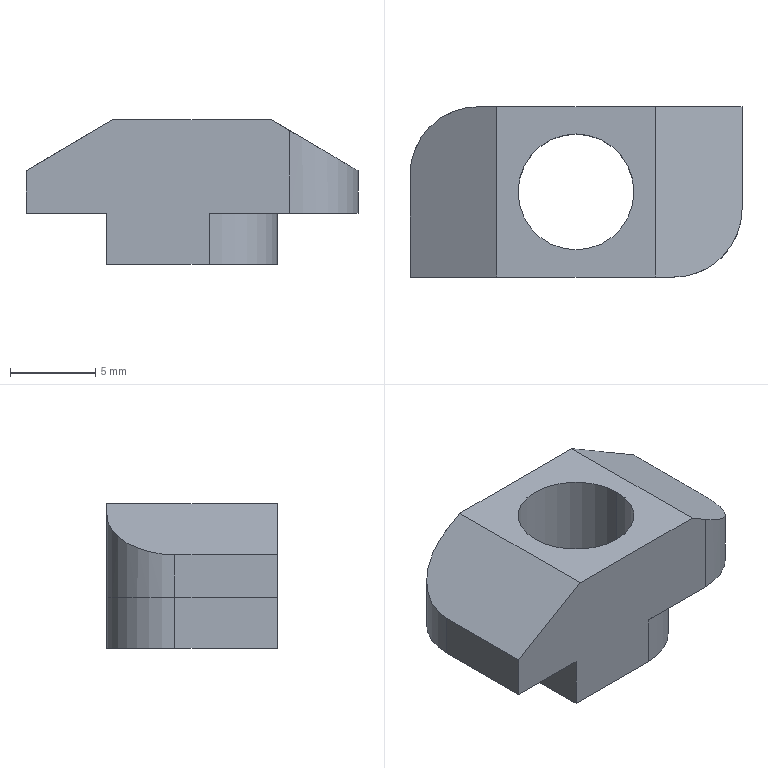Part | NX | features BREP 1 | 1 solid | 18 faces | box 19.5 x 10 x 8.5 mm | volume 869.428 mm3 | plane 12 | cylinder 6 | commonest cylinder face diameters 8 x4 6.8 x2
STEP:
#1=CARTESIAN_POINT('',(-3.4,0.,-8.5));
#2=VERTEX_POINT('',#1);
#3=CARTESIAN_POINT('',(3.4,0.,-8.5));
#4=VERTEX_POINT('',#3);
#5=CARTESIAN_POINT('',(0.,0.,-8.5));
#6=DIRECTION('',(0.,0.,-1.));
#7=DIRECTION('',(-1.,0.,0.));
#8=AXIS2_PLACEMENT_3D('',#5,#6,#7);
#9=CIRCLE('',#8,3.4);
#10=EDGE_CURVE('',#2,#4,#9,.T.);
#11=ORIENTED_EDGE('',*,*,#10,.T.);
#12=CARTESIAN_POINT('',(3.4,0.,0.));
#13=VERTEX_POINT('',#12);
#14=CARTESIAN_POINT('',(3.4,0.,0.));
#15=DIRECTION('',(0.,0.,1.));
#16=VECTOR('',#15,1000.);
#17=LINE('',#14,#16);
#18=EDGE_CURVE('',#4,#13,#17,.T.);
#19=ORIENTED_EDGE('',*,*,#18,.T.);
#20=CARTESIAN_POINT('',(-3.4,0.,0.));
#21=VERTEX_POINT('',#20);
#22=CARTESIAN_POINT('',(0.,0.,0.));
#23=DIRECTION('',(0.,0.,-1.));
#24=DIRECTION('',(-1.,0.,0.));
#25=AXIS2_PLACEMENT_3D('',#22,#23,#24);
#26=CIRCLE('',#25,3.4);
#27=EDGE_CURVE('',#21,#13,#26,.T.);
#28=ORIENTED_EDGE('',*,*,#27,.F.);
#29=CARTESIAN_POINT('',(-3.4,0.,0.));
#30=DIRECTION('',(0.,0.,1.));
#31=VECTOR('',#30,1000.);
#32=LINE('',#29,#31);
#33=EDGE_CURVE('',#2,#21,#32,.T.);
#34=ORIENTED_EDGE('',*,*,#33,.F.);
#35=EDGE_LOOP('',(#11,#19,#28,#34));
#36=FACE_BOUND('',#35,.T.);
#37=CARTESIAN_POINT('',(0.,0.,0.));
#38=DIRECTION('',(0.,0.,1.));
#39=DIRECTION('',(-1.,0.,0.));
#40=AXIS2_PLACEMENT_3D('',#37,#38,#39);
#41=CYLINDRICAL_SURFACE('',#40,3.4);
#42=ADVANCED_FACE('',(#36),#41,.F.);
#43=CARTESIAN_POINT('',(1.,-5.,-5.5));
#44=VERTEX_POINT('',#43);
#45=CARTESIAN_POINT('',(5.75,-5.,-5.5));
#46=VERTEX_POINT('',#45);
#47=CARTESIAN_POINT('',(-9.75,-5.,-5.5));
#48=DIRECTION('',(1.,0.,0.));
#49=VECTOR('',#48,1000.);
#50=LINE('',#47,#49);
#51=EDGE_CURVE('',#44,#46,#50,.T.);
#52=ORIENTED_EDGE('',*,*,#51,.F.);
#53=CARTESIAN_POINT('',(5.,-1.,-5.5));
#54=VERTEX_POINT('',#53);
#55=CARTESIAN_POINT('',(1.,-1.,-5.5));
#56=DIRECTION('',(0.,0.,-1.));
#57=DIRECTION('',(1.,0.,0.));
#58=AXIS2_PLACEMENT_3D('',#55,#56,#57);
#59=CIRCLE('',#58,4.);
#60=EDGE_CURVE('',#54,#44,#59,.T.);
#61=ORIENTED_EDGE('',*,*,#60,.F.);
#62=CARTESIAN_POINT('',(5.,5.,-5.5));
#63=VERTEX_POINT('',#62);
#64=CARTESIAN_POINT('',(5.,-5.,-5.5));
#65=DIRECTION('',(0.,1.,0.));
#66=VECTOR('',#65,1000.);
#67=LINE('',#64,#66);
#68=EDGE_CURVE('',#54,#63,#67,.T.);
#69=ORIENTED_EDGE('',*,*,#68,.T.);
#70=CARTESIAN_POINT('',(9.75,5.,-5.5));
#71=VERTEX_POINT('',#70);
#72=CARTESIAN_POINT('',(-9.75,5.,-5.5));
#73=DIRECTION('',(-1.,0.,0.));
#74=VECTOR('',#73,1000.);
#75=LINE('',#72,#74);
#76=EDGE_CURVE('',#71,#63,#75,.T.);
#77=ORIENTED_EDGE('',*,*,#76,.F.);
#78=CARTESIAN_POINT('',(9.75,-1.,-5.5));
#79=VERTEX_POINT('',#78);
#80=CARTESIAN_POINT('',(9.75,5.,-5.5));
#81=DIRECTION('',(0.,1.,0.));
#82=VECTOR('',#81,1000.);
#83=LINE('',#80,#82);
#84=EDGE_CURVE('',#79,#71,#83,.T.);
#85=ORIENTED_EDGE('',*,*,#84,.F.);
#86=CARTESIAN_POINT('',(5.75,-1.,-5.5));
#87=DIRECTION('',(0.,0.,1.));
#88=DIRECTION('',(1.,0.,0.));
#89=AXIS2_PLACEMENT_3D('',#86,#87,#88);
#90=CIRCLE('',#89,4.);
#91=EDGE_CURVE('',#46,#79,#90,.T.);
#92=ORIENTED_EDGE('',*,*,#91,.F.);
#93=EDGE_LOOP('',(#52,#61,#69,#77,#85,#92));
#94=FACE_BOUND('',#93,.T.);
#95=CARTESIAN_POINT('',(0.,0.,-5.5));
#96=DIRECTION('',(0.,0.,-1.));
#97=DIRECTION('',(0.,-1.,0.));
#98=AXIS2_PLACEMENT_3D('',#95,#96,#97);
#99=PLANE('',#98);
#100=ADVANCED_FACE('',(#94),#99,.T.);
#101=ORIENTED_EDGE('',*,*,#84,.T.);
#102=CARTESIAN_POINT('',(9.75,5.,-3.));
#103=VERTEX_POINT('',#102);
#104=CARTESIAN_POINT('',(9.75,5.,-5.5));
#105=DIRECTION('',(0.,0.,1.));
#106=VECTOR('',#105,1000.);
#107=LINE('',#104,#106);
#108=EDGE_CURVE('',#71,#103,#107,.T.);
#109=ORIENTED_EDGE('',*,*,#108,.T.);
#110=CARTESIAN_POINT('',(9.75,-1.,-3.));
#111=VERTEX_POINT('',#110);
#112=CARTESIAN_POINT('',(9.75,5.,-3.));
#113=DIRECTION('',(0.,1.,0.));
#114=VECTOR('',#113,1000.);
#115=LINE('',#112,#114);
#116=EDGE_CURVE('',#111,#103,#115,.T.);
#117=ORIENTED_EDGE('',*,*,#116,.F.);
#118=CARTESIAN_POINT('',(9.75,-1.,-5.5));
#119=DIRECTION('',(0.,0.,1.));
#120=VECTOR('',#119,1000.);
#121=LINE('',#118,#120);
#122=EDGE_CURVE('',#79,#111,#121,.T.);
#123=ORIENTED_EDGE('',*,*,#122,.F.);
#124=EDGE_LOOP('',(#101,#109,#117,#123));
#125=FACE_BOUND('',#124,.T.);
#126=CARTESIAN_POINT('',(9.75,5.,-5.5));
#127=DIRECTION('',(-1.,0.,0.));
#128=DIRECTION('',(0.,1.,0.));
#129=AXIS2_PLACEMENT_3D('',#126,#127,#128);
#130=PLANE('',#129);
#131=ADVANCED_FACE('',(#125),#130,.F.);
#132=CARTESIAN_POINT('',(-4.65,5.,0.));
#133=VERTEX_POINT('',#132);
#134=CARTESIAN_POINT('',(-5.75,5.,-0.6471));
#135=VERTEX_POINT('',#134);
#136=CARTESIAN_POINT('',(-9.75,5.,-3.));
#137=DIRECTION('',(-0.8619,0.,-0.507));
#138=VECTOR('',#137,1000.);
#139=LINE('',#136,#138);
#140=EDGE_CURVE('',#133,#135,#139,.T.);
#141=ORIENTED_EDGE('',*,*,#140,.F.);
#142=CARTESIAN_POINT('',(4.65,5.,0.));
#143=VERTEX_POINT('',#142);
#144=CARTESIAN_POINT('',(-9.75,5.,0.));
#145=DIRECTION('',(-1.,0.,0.));
#146=VECTOR('',#145,1000.);
#147=LINE('',#144,#146);
#148=EDGE_CURVE('',#143,#133,#147,.T.);
#149=ORIENTED_EDGE('',*,*,#148,.F.);
#150=CARTESIAN_POINT('',(9.75,5.,-3.));
#151=DIRECTION('',(-0.8619,0.,0.507));
#152=VECTOR('',#151,1000.);
#153=LINE('',#150,#152);
#154=EDGE_CURVE('',#103,#143,#153,.T.);
#155=ORIENTED_EDGE('',*,*,#154,.F.);
#156=ORIENTED_EDGE('',*,*,#108,.F.);
#157=ORIENTED_EDGE('',*,*,#76,.T.);
#158=CARTESIAN_POINT('',(5.,5.,-8.5));
#159=VERTEX_POINT('',#158);
#160=CARTESIAN_POINT('',(5.,5.,-8.5));
#161=DIRECTION('',(0.,0.,1.));
#162=VECTOR('',#161,1000.);
#163=LINE('',#160,#162);
#164=EDGE_CURVE('',#159,#63,#163,.T.);
#165=ORIENTED_EDGE('',*,*,#164,.F.);
#166=CARTESIAN_POINT('',(-1.,5.,-8.5));
#167=VERTEX_POINT('',#166);
#168=CARTESIAN_POINT('',(-5.,5.,-8.5));
#169=DIRECTION('',(-1.,0.,0.));
#170=VECTOR('',#169,1000.);
#171=LINE('',#168,#170);
#172=EDGE_CURVE('',#159,#167,#171,.T.);
#173=ORIENTED_EDGE('',*,*,#172,.T.);
#174=CARTESIAN_POINT('',(-1.,5.,-5.5));
#175=VERTEX_POINT('',#174);
#176=CARTESIAN_POINT('',(-1.,5.,-5.5));
#177=DIRECTION('',(0.,0.,-1.));
#178=VECTOR('',#177,1000.);
#179=LINE('',#176,#178);
#180=EDGE_CURVE('',#175,#167,#179,.T.);
#181=ORIENTED_EDGE('',*,*,#180,.F.);
#182=CARTESIAN_POINT('',(-5.75,5.,-5.5));
#183=VERTEX_POINT('',#182);
#184=CARTESIAN_POINT('',(-9.75,5.,-5.5));
#185=DIRECTION('',(-1.,0.,0.));
#186=VECTOR('',#185,1000.);
#187=LINE('',#184,#186);
#188=EDGE_CURVE('',#175,#183,#187,.T.);
#189=ORIENTED_EDGE('',*,*,#188,.T.);
#190=CARTESIAN_POINT('',(-5.75,5.,-5.5));
#191=DIRECTION('',(0.,0.,-1.));
#192=VECTOR('',#191,1000.);
#193=LINE('',#190,#192);
#194=EDGE_CURVE('',#135,#183,#193,.T.);
#195=ORIENTED_EDGE('',*,*,#194,.F.);
#196=EDGE_LOOP('',(#141,#149,#155,#156,#157,#165,#173,#181,#189,#195));
#197=FACE_BOUND('',#196,.T.);
#198=CARTESIAN_POINT('',(-9.75,5.,-5.5));
#199=DIRECTION('',(0.,-1.,0.));
#200=DIRECTION('',(0.,0.,-1.));
#201=AXIS2_PLACEMENT_3D('',#198,#199,#200);
#202=PLANE('',#201);
#203=ADVANCED_FACE('',(#197),#202,.F.);
#204=CARTESIAN_POINT('',(-9.75,1.,-5.5));
#205=VERTEX_POINT('',#204);
#206=CARTESIAN_POINT('',(-9.75,-5.,-5.5));
#207=VERTEX_POINT('',#206);
#208=CARTESIAN_POINT('',(-9.75,5.,-5.5));
#209=DIRECTION('',(0.,-1.,0.));
#210=VECTOR('',#209,1000.);
#211=LINE('',#208,#210);
#212=EDGE_CURVE('',#205,#207,#211,.T.);
#213=ORIENTED_EDGE('',*,*,#212,.T.);
#214=CARTESIAN_POINT('',(-9.75,-5.,-3.));
#215=VERTEX_POINT('',#214);
#216=CARTESIAN_POINT('',(-9.75,-5.,-5.5));
#217=DIRECTION('',(0.,0.,1.));
#218=VECTOR('',#217,1000.);
#219=LINE('',#216,#218);
#220=EDGE_CURVE('',#207,#215,#219,.T.);
#221=ORIENTED_EDGE('',*,*,#220,.T.);
#222=CARTESIAN_POINT('',(-9.75,1.,-3.));
#223=VERTEX_POINT('',#222);
#224=CARTESIAN_POINT('',(-9.75,5.,-3.));
#225=DIRECTION('',(0.,-1.,0.));
#226=VECTOR('',#225,1000.);
#227=LINE('',#224,#226);
#228=EDGE_CURVE('',#223,#215,#227,.T.);
#229=ORIENTED_EDGE('',*,*,#228,.F.);
#230=CARTESIAN_POINT('',(-9.75,1.,-5.5));
#231=DIRECTION('',(0.,0.,1.));
#232=VECTOR('',#231,1000.);
#233=LINE('',#230,#232);
#234=EDGE_CURVE('',#205,#223,#233,.T.);
#235=ORIENTED_EDGE('',*,*,#234,.F.);
#236=EDGE_LOOP('',(#213,#221,#229,#235));
#237=FACE_BOUND('',#236,.T.);
#238=CARTESIAN_POINT('',(-9.75,5.,-5.5));
#239=DIRECTION('',(1.,0.,0.));
#240=DIRECTION('',(0.,1.,0.));
#241=AXIS2_PLACEMENT_3D('',#238,#239,#240);
#242=PLANE('',#241);
#243=ADVANCED_FACE('',(#237),#242,.F.);
#244=CARTESIAN_POINT('',(4.65,-5.,0.));
#245=VERTEX_POINT('',#244);
#246=CARTESIAN_POINT('',(5.75,-5.,-0.6471));
#247=VERTEX_POINT('',#246);
#248=CARTESIAN_POINT('',(9.75,-5.,-3.));
#249=DIRECTION('',(0.8619,0.,-0.507));
#250=VECTOR('',#249,1000.);
#251=LINE('',#248,#250);
#252=EDGE_CURVE('',#245,#247,#251,.T.);
#253=ORIENTED_EDGE('',*,*,#252,.F.);
#254=CARTESIAN_POINT('',(-4.65,-5.,0.));
#255=VERTEX_POINT('',#254);
#256=CARTESIAN_POINT('',(-9.75,-5.,0.));
#257=DIRECTION('',(1.,0.,0.));
#258=VECTOR('',#257,1000.);
#259=LINE('',#256,#258);
#260=EDGE_CURVE('',#255,#245,#259,.T.);
#261=ORIENTED_EDGE('',*,*,#260,.F.);
#262=CARTESIAN_POINT('',(-9.75,-5.,-3.));
#263=DIRECTION('',(0.8619,0.,0.507));
#264=VECTOR('',#263,1000.);
#265=LINE('',#262,#264);
#266=EDGE_CURVE('',#215,#255,#265,.T.);
#267=ORIENTED_EDGE('',*,*,#266,.F.);
#268=ORIENTED_EDGE('',*,*,#220,.F.);
#269=CARTESIAN_POINT('',(-5.,-5.,-5.5));
#270=VERTEX_POINT('',#269);
#271=CARTESIAN_POINT('',(-9.75,-5.,-5.5));
#272=DIRECTION('',(1.,0.,0.));
#273=VECTOR('',#272,1000.);
#274=LINE('',#271,#273);
#275=EDGE_CURVE('',#207,#270,#274,.T.);
#276=ORIENTED_EDGE('',*,*,#275,.T.);
#277=CARTESIAN_POINT('',(-5.,-5.,-8.5));
#278=VERTEX_POINT('',#277);
#279=CARTESIAN_POINT('',(-5.,-5.,-8.5));
#280=DIRECTION('',(0.,0.,1.));
#281=VECTOR('',#280,1000.);
#282=LINE('',#279,#281);
#283=EDGE_CURVE('',#278,#270,#282,.T.);
#284=ORIENTED_EDGE('',*,*,#283,.F.);
#285=CARTESIAN_POINT('',(1.,-5.,-8.5));
#286=VERTEX_POINT('',#285);
#287=CARTESIAN_POINT('',(-5.,-5.,-8.5));
#288=DIRECTION('',(1.,0.,0.));
#289=VECTOR('',#288,1000.);
#290=LINE('',#287,#289);
#291=EDGE_CURVE('',#278,#286,#290,.T.);
#292=ORIENTED_EDGE('',*,*,#291,.T.);
#293=CARTESIAN_POINT('',(1.,-5.,-5.5));
#294=DIRECTION('',(0.,0.,-1.));
#295=VECTOR('',#294,1000.);
#296=LINE('',#293,#295);
#297=EDGE_CURVE('',#44,#286,#296,.T.);
#298=ORIENTED_EDGE('',*,*,#297,.F.);
#299=ORIENTED_EDGE('',*,*,#51,.T.);
#300=CARTESIAN_POINT('',(5.75,-5.,-5.5));
#301=DIRECTION('',(0.,0.,-1.));
#302=VECTOR('',#301,1000.);
#303=LINE('',#300,#302);
#304=EDGE_CURVE('',#247,#46,#303,.T.);
#305=ORIENTED_EDGE('',*,*,#304,.F.);
#306=EDGE_LOOP('',(#253,#261,#267,#268,#276,#284,#292,#298,#299,#305));
#307=FACE_BOUND('',#306,.T.);
#308=CARTESIAN_POINT('',(-9.75,-5.,-5.5));
#309=DIRECTION('',(0.,1.,0.));
#310=DIRECTION('',(1.,0.,0.));
#311=AXIS2_PLACEMENT_3D('',#308,#309,#310);
#312=PLANE('',#311);
#313=ADVANCED_FACE('',(#307),#312,.F.);
#314=ORIENTED_EDGE('',*,*,#188,.F.);
#315=CARTESIAN_POINT('',(-5.,1.,-5.5));
#316=VERTEX_POINT('',#315);
#317=CARTESIAN_POINT('',(-1.,1.,-5.5));
#318=DIRECTION('',(0.,0.,-1.));
#319=DIRECTION('',(1.,0.,0.));
#320=AXIS2_PLACEMENT_3D('',#317,#318,#319);
#321=CIRCLE('',#320,4.);
#322=EDGE_CURVE('',#316,#175,#321,.T.);
#323=ORIENTED_EDGE('',*,*,#322,.F.);
#324=CARTESIAN_POINT('',(-5.,-5.,-5.5));
#325=DIRECTION('',(0.,-1.,0.));
#326=VECTOR('',#325,1000.);
#327=LINE('',#324,#326);
#328=EDGE_CURVE('',#316,#270,#327,.T.);
#329=ORIENTED_EDGE('',*,*,#328,.T.);
#330=ORIENTED_EDGE('',*,*,#275,.F.);
#331=ORIENTED_EDGE('',*,*,#212,.F.);
#332=CARTESIAN_POINT('',(-5.75,1.,-5.5));
#333=DIRECTION('',(0.,0.,1.));
#334=DIRECTION('',(1.,0.,0.));
#335=AXIS2_PLACEMENT_3D('',#332,#333,#334);
#336=CIRCLE('',#335,4.);
#337=EDGE_CURVE('',#183,#205,#336,.T.);
#338=ORIENTED_EDGE('',*,*,#337,.F.);
#339=EDGE_LOOP('',(#314,#323,#329,#330,#331,#338));
#340=FACE_BOUND('',#339,.T.);
#341=CARTESIAN_POINT('',(0.,0.,-5.5));
#342=DIRECTION('',(0.,0.,-1.));
#343=DIRECTION('',(0.,-1.,0.));
#344=AXIS2_PLACEMENT_3D('',#341,#342,#343);
#345=PLANE('',#344);
#346=ADVANCED_FACE('',(#340),#345,.T.);
#347=ORIENTED_EDGE('',*,*,#148,.T.);
#348=CARTESIAN_POINT('',(-4.65,0.,0.));
#349=DIRECTION('',(0.,1.,0.));
#350=VECTOR('',#349,1000.);
#351=LINE('',#348,#350);
#352=EDGE_CURVE('',#255,#133,#351,.T.);
#353=ORIENTED_EDGE('',*,*,#352,.F.);
#354=ORIENTED_EDGE('',*,*,#260,.T.);
#355=CARTESIAN_POINT('',(4.65,0.,0.));
#356=DIRECTION('',(0.,-1.,0.));
#357=VECTOR('',#356,1000.);
#358=LINE('',#355,#357);
#359=EDGE_CURVE('',#143,#245,#358,.T.);
#360=ORIENTED_EDGE('',*,*,#359,.F.);
#361=EDGE_LOOP('',(#347,#353,#354,#360));
#362=FACE_BOUND('',#361,.T.);
#363=ORIENTED_EDGE('',*,*,#27,.T.);
#364=CARTESIAN_POINT('',(0.,0.,0.));
#365=DIRECTION('',(0.,0.,-1.));
#366=DIRECTION('',(-1.,0.,0.));
#367=AXIS2_PLACEMENT_3D('',#364,#365,#366);
#368=CIRCLE('',#367,3.4);
#369=EDGE_CURVE('',#13,#21,#368,.T.);
#370=ORIENTED_EDGE('',*,*,#369,.T.);
#371=EDGE_LOOP('',(#363,#370));
#372=FACE_BOUND('',#371,.T.);
#373=CARTESIAN_POINT('',(0.,0.,0.));
#374=DIRECTION('',(0.,0.,-1.));
#375=DIRECTION('',(0.,-1.,0.));
#376=AXIS2_PLACEMENT_3D('',#373,#374,#375);
#377=PLANE('',#376);
#378=ADVANCED_FACE('',(#362,#372),#377,.F.);
#379=CARTESIAN_POINT('',(5.,-1.,-8.5));
#380=VERTEX_POINT('',#379);
#381=CARTESIAN_POINT('',(5.,-5.,-8.5));
#382=DIRECTION('',(0.,1.,0.));
#383=VECTOR('',#382,1000.);
#384=LINE('',#381,#383);
#385=EDGE_CURVE('',#380,#159,#384,.T.);
#386=ORIENTED_EDGE('',*,*,#385,.T.);
#387=ORIENTED_EDGE('',*,*,#164,.T.);
#388=ORIENTED_EDGE('',*,*,#68,.F.);
#389=CARTESIAN_POINT('',(5.,-1.,-8.5));
#390=DIRECTION('',(0.,0.,1.));
#391=VECTOR('',#390,1000.);
#392=LINE('',#389,#391);
#393=EDGE_CURVE('',#380,#54,#392,.T.);
#394=ORIENTED_EDGE('',*,*,#393,.F.);
#395=EDGE_LOOP('',(#386,#387,#388,#394));
#396=FACE_BOUND('',#395,.T.);
#397=CARTESIAN_POINT('',(5.,-5.,-8.5));
#398=DIRECTION('',(-1.,0.,0.));
#399=DIRECTION('',(0.,0.,1.));
#400=AXIS2_PLACEMENT_3D('',#397,#398,#399);
#401=PLANE('',#400);
#402=ADVANCED_FACE('',(#396),#401,.F.);
#403=CARTESIAN_POINT('',(-5.,1.,-8.5));
#404=VERTEX_POINT('',#403);
#405=CARTESIAN_POINT('',(-5.,-5.,-8.5));
#406=DIRECTION('',(0.,-1.,0.));
#407=VECTOR('',#406,1000.);
#408=LINE('',#405,#407);
#409=EDGE_CURVE('',#404,#278,#408,.T.);
#410=ORIENTED_EDGE('',*,*,#409,.T.);
#411=ORIENTED_EDGE('',*,*,#283,.T.);
#412=ORIENTED_EDGE('',*,*,#328,.F.);
#413=CARTESIAN_POINT('',(-5.,1.,-8.5));
#414=DIRECTION('',(0.,0.,1.));
#415=VECTOR('',#414,1000.);
#416=LINE('',#413,#415);
#417=EDGE_CURVE('',#404,#316,#416,.T.);
#418=ORIENTED_EDGE('',*,*,#417,.F.);
#419=EDGE_LOOP('',(#410,#411,#412,#418));
#420=FACE_BOUND('',#419,.T.);
#421=CARTESIAN_POINT('',(-5.,-5.,-8.5));
#422=DIRECTION('',(1.,0.,0.));
#423=DIRECTION('',(0.,1.,0.));
#424=AXIS2_PLACEMENT_3D('',#421,#422,#423);
#425=PLANE('',#424);
#426=ADVANCED_FACE('',(#420),#425,.F.);
#427=ORIENTED_EDGE('',*,*,#291,.F.);
#428=ORIENTED_EDGE('',*,*,#409,.F.);
#429=CARTESIAN_POINT('',(-1.,1.,-8.5));
#430=DIRECTION('',(0.,0.,1.));
#431=DIRECTION('',(-1.,0.,0.));
#432=AXIS2_PLACEMENT_3D('',#429,#430,#431);
#433=CIRCLE('',#432,4.);
#434=EDGE_CURVE('',#167,#404,#433,.T.);
#435=ORIENTED_EDGE('',*,*,#434,.F.);
#436=ORIENTED_EDGE('',*,*,#172,.F.);
#437=ORIENTED_EDGE('',*,*,#385,.F.);
#438=CARTESIAN_POINT('',(1.,-1.,-8.5));
#439=DIRECTION('',(0.,0.,1.));
#440=DIRECTION('',(-1.,0.,0.));
#441=AXIS2_PLACEMENT_3D('',#438,#439,#440);
#442=CIRCLE('',#441,4.);
#443=EDGE_CURVE('',#286,#380,#442,.T.);
#444=ORIENTED_EDGE('',*,*,#443,.F.);
#445=EDGE_LOOP('',(#427,#428,#435,#436,#437,#444));
#446=FACE_BOUND('',#445,.T.);
#447=ORIENTED_EDGE('',*,*,#10,.F.);
#448=CARTESIAN_POINT('',(0.,0.,-8.5));
#449=DIRECTION('',(0.,0.,-1.));
#450=DIRECTION('',(-1.,0.,0.));
#451=AXIS2_PLACEMENT_3D('',#448,#449,#450);
#452=CIRCLE('',#451,3.4);
#453=EDGE_CURVE('',#4,#2,#452,.T.);
#454=ORIENTED_EDGE('',*,*,#453,.F.);
#455=EDGE_LOOP('',(#447,#454));
#456=FACE_BOUND('',#455,.T.);
#457=CARTESIAN_POINT('',(0.,0.,-8.5));
#458=DIRECTION('',(0.,0.,1.));
#459=DIRECTION('',(1.,0.,0.));
#460=AXIS2_PLACEMENT_3D('',#457,#458,#459);
#461=PLANE('',#460);
#462=ADVANCED_FACE('',(#446,#456),#461,.F.);
#463=ORIENTED_EDGE('',*,*,#18,.F.);
#464=ORIENTED_EDGE('',*,*,#453,.T.);
#465=ORIENTED_EDGE('',*,*,#33,.T.);
#466=ORIENTED_EDGE('',*,*,#369,.F.);
#467=EDGE_LOOP('',(#463,#464,#465,#466));
#468=FACE_BOUND('',#467,.T.);
#469=CARTESIAN_POINT('',(0.,0.,0.));
#470=DIRECTION('',(0.,0.,1.));
#471=DIRECTION('',(-1.,0.,0.));
#472=AXIS2_PLACEMENT_3D('',#469,#470,#471);
#473=CYLINDRICAL_SURFACE('',#472,3.4);
#474=ADVANCED_FACE('',(#468),#473,.F.);
#475=ORIENTED_EDGE('',*,*,#116,.T.);
#476=ORIENTED_EDGE('',*,*,#154,.T.);
#477=ORIENTED_EDGE('',*,*,#359,.T.);
#478=ORIENTED_EDGE('',*,*,#252,.T.);
#479=CARTESIAN_POINT('',(9.75,-1.,-3.));
#480=CARTESIAN_POINT('',(9.75,-3.343,-3.));
#481=CARTESIAN_POINT('',(8.093,-5.,-2.025));
#482=CARTESIAN_POINT('',(5.75,-5.,-0.6471));
#483=(BOUNDED_CURVE()B_SPLINE_CURVE(3,(#479,#480,#481,#482),.UNSPECIFIED.,.F.,.F.)B_SPLINE_CURVE_WITH_KNOTS((4,4),(3.142,4.712),.UNSPECIFIED.)CURVE()GEOMETRIC_REPRESENTATION_ITEM()RATIONAL_B_SPLINE_CURVE((1.,0.8047,0.8047,1.))REPRESENTATION_ITEM(''));
#484=EDGE_CURVE('',#111,#247,#483,.T.);
#485=ORIENTED_EDGE('',*,*,#484,.F.);
#486=EDGE_LOOP('',(#475,#476,#477,#478,#485));
#487=FACE_BOUND('',#486,.T.);
#488=CARTESIAN_POINT('',(9.75,5.,-3.));
#489=DIRECTION('',(-0.507,0.,-0.8619));
#490=DIRECTION('',(-0.8619,0.,0.507));
#491=AXIS2_PLACEMENT_3D('',#488,#489,#490);
#492=PLANE('',#491);
#493=ADVANCED_FACE('',(#487),#492,.F.);
#494=ORIENTED_EDGE('',*,*,#228,.T.);
#495=ORIENTED_EDGE('',*,*,#266,.T.);
#496=ORIENTED_EDGE('',*,*,#352,.T.);
#497=ORIENTED_EDGE('',*,*,#140,.T.);
#498=CARTESIAN_POINT('',(-9.75,1.,-3.));
#499=CARTESIAN_POINT('',(-9.75,3.343,-3.));
#500=CARTESIAN_POINT('',(-8.093,5.,-2.025));
#501=CARTESIAN_POINT('',(-5.75,5.,-0.6471));
#502=(BOUNDED_CURVE()B_SPLINE_CURVE(3,(#498,#499,#500,#501),.UNSPECIFIED.,.F.,.F.)B_SPLINE_CURVE_WITH_KNOTS((4,4),(3.142,4.712),.UNSPECIFIED.)CURVE()GEOMETRIC_REPRESENTATION_ITEM()RATIONAL_B_SPLINE_CURVE((1.,0.8047,0.8047,1.))REPRESENTATION_ITEM(''));
#503=EDGE_CURVE('',#223,#135,#502,.T.);
#504=ORIENTED_EDGE('',*,*,#503,.F.);
#505=EDGE_LOOP('',(#494,#495,#496,#497,#504));
#506=FACE_BOUND('',#505,.T.);
#507=CARTESIAN_POINT('',(-9.75,5.,-3.));
#508=DIRECTION('',(0.507,0.,-0.8619));
#509=DIRECTION('',(0.,-1.,0.));
#510=AXIS2_PLACEMENT_3D('',#507,#508,#509);
#511=PLANE('',#510);
#512=ADVANCED_FACE('',(#506),#511,.F.);
#513=ORIENTED_EDGE('',*,*,#443,.T.);
#514=ORIENTED_EDGE('',*,*,#393,.T.);
#515=ORIENTED_EDGE('',*,*,#60,.T.);
#516=ORIENTED_EDGE('',*,*,#297,.T.);
#517=EDGE_LOOP('',(#513,#514,#515,#516));
#518=FACE_BOUND('',#517,.T.);
#519=CARTESIAN_POINT('',(1.,-1.,-8.5));
#520=DIRECTION('',(0.,0.,1.));
#521=DIRECTION('',(-1.,0.,0.));
#522=AXIS2_PLACEMENT_3D('',#519,#520,#521);
#523=CYLINDRICAL_SURFACE('',#522,4.);
#524=ADVANCED_FACE('',(#518),#523,.T.);
#525=ORIENTED_EDGE('',*,*,#434,.T.);
#526=ORIENTED_EDGE('',*,*,#417,.T.);
#527=ORIENTED_EDGE('',*,*,#322,.T.);
#528=ORIENTED_EDGE('',*,*,#180,.T.);
#529=EDGE_LOOP('',(#525,#526,#527,#528));
#530=FACE_BOUND('',#529,.T.);
#531=CARTESIAN_POINT('',(-1.,1.,-8.5));
#532=DIRECTION('',(0.,0.,1.));
#533=DIRECTION('',(-1.,0.,0.));
#534=AXIS2_PLACEMENT_3D('',#531,#532,#533);
#535=CYLINDRICAL_SURFACE('',#534,4.);
#536=ADVANCED_FACE('',(#530),#535,.T.);
#537=ORIENTED_EDGE('',*,*,#91,.T.);
#538=ORIENTED_EDGE('',*,*,#122,.T.);
#539=ORIENTED_EDGE('',*,*,#484,.T.);
#540=ORIENTED_EDGE('',*,*,#304,.T.);
#541=EDGE_LOOP('',(#537,#538,#539,#540));
#542=FACE_BOUND('',#541,.T.);
#543=CARTESIAN_POINT('',(5.75,-1.,-5.5));
#544=DIRECTION('',(0.,0.,1.));
#545=DIRECTION('',(-1.,0.,0.));
#546=AXIS2_PLACEMENT_3D('',#543,#544,#545);
#547=CYLINDRICAL_SURFACE('',#546,4.);
#548=ADVANCED_FACE('',(#542),#547,.T.);
#549=ORIENTED_EDGE('',*,*,#337,.T.);
#550=ORIENTED_EDGE('',*,*,#234,.T.);
#551=ORIENTED_EDGE('',*,*,#503,.T.);
#552=ORIENTED_EDGE('',*,*,#194,.T.);
#553=EDGE_LOOP('',(#549,#550,#551,#552));
#554=FACE_BOUND('',#553,.T.);
#555=CARTESIAN_POINT('',(-5.75,1.,-5.5));
#556=DIRECTION('',(0.,0.,1.));
#557=DIRECTION('',(-1.,0.,0.));
#558=AXIS2_PLACEMENT_3D('',#555,#556,#557);
#559=CYLINDRICAL_SURFACE('',#558,4.);
#560=ADVANCED_FACE('',(#554),#559,.T.);
#561=CLOSED_SHELL('',(#42,#100,#131,#203,#243,#313,#346,#378,#402,#426,#462,#474,#493,#512,#524,#536,#548,#560));
#562=MANIFOLD_SOLID_BREP('',#561);
#563=(LENGTH_UNIT()NAMED_UNIT(*)SI_UNIT(.MILLI.,.METRE.));
#564=UNCERTAINTY_MEASURE_WITH_UNIT(LENGTH_MEASURE(0.00001),#563,'','');
#565=(NAMED_UNIT(*)PLANE_ANGLE_UNIT()SI_UNIT($,.RADIAN.));
#566=(NAMED_UNIT(*)SI_UNIT($,.STERADIAN.)SOLID_ANGLE_UNIT());
#567=(GEOMETRIC_REPRESENTATION_CONTEXT(3)GLOBAL_UNCERTAINTY_ASSIGNED_CONTEXT((#564))GLOBAL_UNIT_ASSIGNED_CONTEXT((#563,#565,#566))REPRESENTATION_CONTEXT('',''));
#568=ADVANCED_BREP_SHAPE_REPRESENTATION('',(#562),#567);